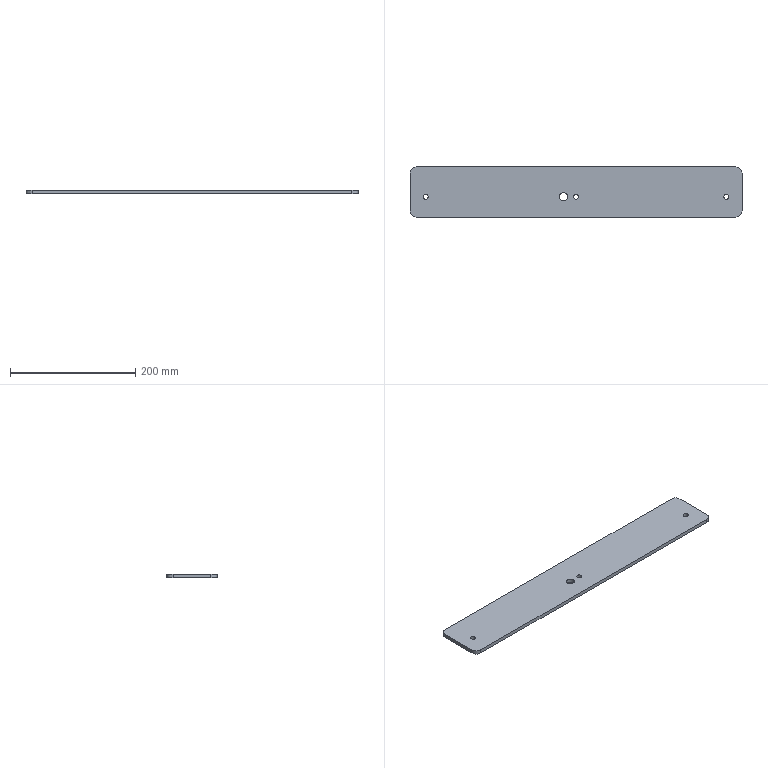Part | SolidWorks | features FlatPattern 1, SMBaseFlange 1, SheetMetal 1 | 1 solid | 18 faces | box 530 x 80 x 6 mm | volume 252184 mm3 | cylinder 12 | plane 6 | commonest cylinder face diameters 8 x6 20 x4 13 x2
STEP:
#1=CARTESIAN_POINT('',(-234.,927.5,6.));
#2=VERTEX_POINT('',#1);
#3=CARTESIAN_POINT('',(-226.,927.5,6.));
#4=VERTEX_POINT('',#3);
#5=CARTESIAN_POINT('',(-230.,927.5,6.));
#6=DIRECTION('',(0.,0.,1.));
#7=DIRECTION('',(1.,0.,0.));
#8=AXIS2_PLACEMENT_3D('',#5,#6,#7);
#9=CIRCLE('',#8,4.);
#10=EDGE_CURVE('',#2,#4,#9,.T.);
#11=ORIENTED_EDGE('',*,*,#10,.T.);
#12=CARTESIAN_POINT('',(-226.,927.5,0.));
#13=VERTEX_POINT('',#12);
#14=CARTESIAN_POINT('',(-226.,927.5,6.));
#15=DIRECTION('',(0.,0.,-1.));
#16=VECTOR('',#15,1000.);
#17=LINE('',#14,#16);
#18=EDGE_CURVE('',#4,#13,#17,.T.);
#19=ORIENTED_EDGE('',*,*,#18,.T.);
#20=CARTESIAN_POINT('',(-234.,927.5,0.));
#21=VERTEX_POINT('',#20);
#22=CARTESIAN_POINT('',(-230.,927.5,0.));
#23=DIRECTION('',(0.,0.,1.));
#24=DIRECTION('',(1.,0.,0.));
#25=AXIS2_PLACEMENT_3D('',#22,#23,#24);
#26=CIRCLE('',#25,4.);
#27=EDGE_CURVE('',#21,#13,#26,.T.);
#28=ORIENTED_EDGE('',*,*,#27,.F.);
#29=CARTESIAN_POINT('',(-234.,927.5,6.));
#30=DIRECTION('',(0.,0.,-1.));
#31=VECTOR('',#30,1000.);
#32=LINE('',#29,#31);
#33=EDGE_CURVE('',#2,#21,#32,.T.);
#34=ORIENTED_EDGE('',*,*,#33,.F.);
#35=EDGE_LOOP('',(#11,#19,#28,#34));
#36=FACE_OUTER_BOUND('',#35,.T.);
#37=CARTESIAN_POINT('',(-230.,927.5,6.));
#38=DIRECTION('',(0.,0.,-1.));
#39=DIRECTION('',(-1.,0.,0.));
#40=AXIS2_PLACEMENT_3D('',#37,#38,#39);
#41=CYLINDRICAL_SURFACE('',#40,4.);
#42=ADVANCED_FACE('',(#36),#41,.F.);
#43=CARTESIAN_POINT('',(-16.5,927.5,6.));
#44=VERTEX_POINT('',#43);
#45=CARTESIAN_POINT('',(-3.5,927.5,6.));
#46=VERTEX_POINT('',#45);
#47=CARTESIAN_POINT('',(-10.,927.5,6.));
#48=DIRECTION('',(0.,0.,1.));
#49=DIRECTION('',(1.,0.,0.));
#50=AXIS2_PLACEMENT_3D('',#47,#48,#49);
#51=CIRCLE('',#50,6.5);
#52=EDGE_CURVE('',#44,#46,#51,.T.);
#53=ORIENTED_EDGE('',*,*,#52,.T.);
#54=CARTESIAN_POINT('',(-3.5,927.5,0.));
#55=VERTEX_POINT('',#54);
#56=CARTESIAN_POINT('',(-3.5,927.5,6.));
#57=DIRECTION('',(0.,0.,-1.));
#58=VECTOR('',#57,1000.);
#59=LINE('',#56,#58);
#60=EDGE_CURVE('',#46,#55,#59,.T.);
#61=ORIENTED_EDGE('',*,*,#60,.T.);
#62=CARTESIAN_POINT('',(-16.5,927.5,0.));
#63=VERTEX_POINT('',#62);
#64=CARTESIAN_POINT('',(-10.,927.5,0.));
#65=DIRECTION('',(0.,0.,1.));
#66=DIRECTION('',(1.,0.,0.));
#67=AXIS2_PLACEMENT_3D('',#64,#65,#66);
#68=CIRCLE('',#67,6.5);
#69=EDGE_CURVE('',#63,#55,#68,.T.);
#70=ORIENTED_EDGE('',*,*,#69,.F.);
#71=CARTESIAN_POINT('',(-16.5,927.5,6.));
#72=DIRECTION('',(0.,0.,-1.));
#73=VECTOR('',#72,1000.);
#74=LINE('',#71,#73);
#75=EDGE_CURVE('',#44,#63,#74,.T.);
#76=ORIENTED_EDGE('',*,*,#75,.F.);
#77=EDGE_LOOP('',(#53,#61,#70,#76));
#78=FACE_OUTER_BOUND('',#77,.T.);
#79=CARTESIAN_POINT('',(-10.,927.5,6.));
#80=DIRECTION('',(0.,0.,-1.));
#81=DIRECTION('',(-1.,0.,0.));
#82=AXIS2_PLACEMENT_3D('',#79,#80,#81);
#83=CYLINDRICAL_SURFACE('',#82,6.5);
#84=ADVANCED_FACE('',(#78),#83,.F.);
#85=CARTESIAN_POINT('',(6.,927.5,6.));
#86=VERTEX_POINT('',#85);
#87=CARTESIAN_POINT('',(14.,927.5,6.));
#88=VERTEX_POINT('',#87);
#89=CARTESIAN_POINT('',(10.,927.5,6.));
#90=DIRECTION('',(0.,0.,1.));
#91=DIRECTION('',(1.,0.,0.));
#92=AXIS2_PLACEMENT_3D('',#89,#90,#91);
#93=CIRCLE('',#92,4.);
#94=EDGE_CURVE('',#86,#88,#93,.T.);
#95=ORIENTED_EDGE('',*,*,#94,.T.);
#96=CARTESIAN_POINT('',(14.,927.5,0.));
#97=VERTEX_POINT('',#96);
#98=CARTESIAN_POINT('',(14.,927.5,6.));
#99=DIRECTION('',(0.,0.,-1.));
#100=VECTOR('',#99,1000.);
#101=LINE('',#98,#100);
#102=EDGE_CURVE('',#88,#97,#101,.T.);
#103=ORIENTED_EDGE('',*,*,#102,.T.);
#104=CARTESIAN_POINT('',(6.,927.5,0.));
#105=VERTEX_POINT('',#104);
#106=CARTESIAN_POINT('',(10.,927.5,0.));
#107=DIRECTION('',(0.,0.,1.));
#108=DIRECTION('',(1.,0.,0.));
#109=AXIS2_PLACEMENT_3D('',#106,#107,#108);
#110=CIRCLE('',#109,4.);
#111=EDGE_CURVE('',#105,#97,#110,.T.);
#112=ORIENTED_EDGE('',*,*,#111,.F.);
#113=CARTESIAN_POINT('',(6.,927.5,6.));
#114=DIRECTION('',(0.,0.,-1.));
#115=VECTOR('',#114,1000.);
#116=LINE('',#113,#115);
#117=EDGE_CURVE('',#86,#105,#116,.T.);
#118=ORIENTED_EDGE('',*,*,#117,.F.);
#119=EDGE_LOOP('',(#95,#103,#112,#118));
#120=FACE_OUTER_BOUND('',#119,.T.);
#121=CARTESIAN_POINT('',(10.,927.5,6.));
#122=DIRECTION('',(0.,0.,-1.));
#123=DIRECTION('',(-1.,0.,0.));
#124=AXIS2_PLACEMENT_3D('',#121,#122,#123);
#125=CYLINDRICAL_SURFACE('',#124,4.);
#126=ADVANCED_FACE('',(#120),#125,.F.);
#127=CARTESIAN_POINT('',(246.,927.5,6.));
#128=VERTEX_POINT('',#127);
#129=CARTESIAN_POINT('',(254.,927.5,6.));
#130=VERTEX_POINT('',#129);
#131=CARTESIAN_POINT('',(250.,927.5,6.));
#132=DIRECTION('',(0.,0.,1.));
#133=DIRECTION('',(1.,0.,0.));
#134=AXIS2_PLACEMENT_3D('',#131,#132,#133);
#135=CIRCLE('',#134,4.);
#136=EDGE_CURVE('',#128,#130,#135,.T.);
#137=ORIENTED_EDGE('',*,*,#136,.T.);
#138=CARTESIAN_POINT('',(254.,927.5,0.));
#139=VERTEX_POINT('',#138);
#140=CARTESIAN_POINT('',(254.,927.5,6.));
#141=DIRECTION('',(0.,0.,-1.));
#142=VECTOR('',#141,1000.);
#143=LINE('',#140,#142);
#144=EDGE_CURVE('',#130,#139,#143,.T.);
#145=ORIENTED_EDGE('',*,*,#144,.T.);
#146=CARTESIAN_POINT('',(246.,927.5,0.));
#147=VERTEX_POINT('',#146);
#148=CARTESIAN_POINT('',(250.,927.5,0.));
#149=DIRECTION('',(0.,0.,1.));
#150=DIRECTION('',(1.,0.,0.));
#151=AXIS2_PLACEMENT_3D('',#148,#149,#150);
#152=CIRCLE('',#151,4.);
#153=EDGE_CURVE('',#147,#139,#152,.T.);
#154=ORIENTED_EDGE('',*,*,#153,.F.);
#155=CARTESIAN_POINT('',(246.,927.5,6.));
#156=DIRECTION('',(0.,0.,-1.));
#157=VECTOR('',#156,1000.);
#158=LINE('',#155,#157);
#159=EDGE_CURVE('',#128,#147,#158,.T.);
#160=ORIENTED_EDGE('',*,*,#159,.F.);
#161=EDGE_LOOP('',(#137,#145,#154,#160));
#162=FACE_OUTER_BOUND('',#161,.T.);
#163=CARTESIAN_POINT('',(250.,927.5,6.));
#164=DIRECTION('',(0.,0.,-1.));
#165=DIRECTION('',(-1.,0.,0.));
#166=AXIS2_PLACEMENT_3D('',#163,#164,#165);
#167=CYLINDRICAL_SURFACE('',#166,4.);
#168=ADVANCED_FACE('',(#162),#167,.F.);
#169=CARTESIAN_POINT('',(-255.,905.,6.));
#170=VERTEX_POINT('',#169);
#171=CARTESIAN_POINT('',(-245.,895.,6.));
#172=VERTEX_POINT('',#171);
#173=CARTESIAN_POINT('',(-245.,905.,6.));
#174=DIRECTION('',(0.,0.,1.));
#175=DIRECTION('',(-1.,0.,0.));
#176=AXIS2_PLACEMENT_3D('',#173,#174,#175);
#177=CIRCLE('',#176,10.);
#178=EDGE_CURVE('',#170,#172,#177,.T.);
#179=ORIENTED_EDGE('',*,*,#178,.T.);
#180=CARTESIAN_POINT('',(265.,895.,6.));
#181=VERTEX_POINT('',#180);
#182=CARTESIAN_POINT('',(265.,895.,6.));
#183=DIRECTION('',(1.,0.,0.));
#184=VECTOR('',#183,1000.);
#185=LINE('',#182,#184);
#186=EDGE_CURVE('',#172,#181,#185,.T.);
#187=ORIENTED_EDGE('',*,*,#186,.T.);
#188=CARTESIAN_POINT('',(275.,905.,6.));
#189=VERTEX_POINT('',#188);
#190=CARTESIAN_POINT('',(265.,905.,6.));
#191=DIRECTION('',(0.,0.,1.));
#192=DIRECTION('',(-1.,0.,0.));
#193=AXIS2_PLACEMENT_3D('',#190,#191,#192);
#194=CIRCLE('',#193,10.);
#195=EDGE_CURVE('',#181,#189,#194,.T.);
#196=ORIENTED_EDGE('',*,*,#195,.T.);
#197=CARTESIAN_POINT('',(275.,965.,6.));
#198=VERTEX_POINT('',#197);
#199=CARTESIAN_POINT('',(275.,965.,6.));
#200=DIRECTION('',(0.,1.,0.));
#201=VECTOR('',#200,1000.);
#202=LINE('',#199,#201);
#203=EDGE_CURVE('',#189,#198,#202,.T.);
#204=ORIENTED_EDGE('',*,*,#203,.T.);
#205=CARTESIAN_POINT('',(265.,975.,6.));
#206=VERTEX_POINT('',#205);
#207=CARTESIAN_POINT('',(265.,965.,6.));
#208=DIRECTION('',(0.,0.,1.));
#209=DIRECTION('',(-1.,0.,0.));
#210=AXIS2_PLACEMENT_3D('',#207,#208,#209);
#211=CIRCLE('',#210,10.);
#212=EDGE_CURVE('',#198,#206,#211,.T.);
#213=ORIENTED_EDGE('',*,*,#212,.T.);
#214=CARTESIAN_POINT('',(-245.,975.,6.));
#215=VERTEX_POINT('',#214);
#216=CARTESIAN_POINT('',(265.,975.,6.));
#217=DIRECTION('',(-1.,0.,0.));
#218=VECTOR('',#217,1000.);
#219=LINE('',#216,#218);
#220=EDGE_CURVE('',#206,#215,#219,.T.);
#221=ORIENTED_EDGE('',*,*,#220,.T.);
#222=CARTESIAN_POINT('',(-255.,965.,6.));
#223=VERTEX_POINT('',#222);
#224=CARTESIAN_POINT('',(-245.,965.,6.));
#225=DIRECTION('',(0.,0.,1.));
#226=DIRECTION('',(1.,0.,0.));
#227=AXIS2_PLACEMENT_3D('',#224,#225,#226);
#228=CIRCLE('',#227,10.);
#229=EDGE_CURVE('',#215,#223,#228,.T.);
#230=ORIENTED_EDGE('',*,*,#229,.T.);
#231=CARTESIAN_POINT('',(-255.,965.,6.));
#232=DIRECTION('',(0.,-1.,0.));
#233=VECTOR('',#232,1000.);
#234=LINE('',#231,#233);
#235=EDGE_CURVE('',#223,#170,#234,.T.);
#236=ORIENTED_EDGE('',*,*,#235,.T.);
#237=EDGE_LOOP('',(#179,#187,#196,#204,#213,#221,#230,#236));
#238=FACE_OUTER_BOUND('',#237,.T.);
#239=ORIENTED_EDGE('',*,*,#136,.F.);
#240=CARTESIAN_POINT('',(250.,927.5,6.));
#241=DIRECTION('',(0.,0.,1.));
#242=DIRECTION('',(1.,0.,0.));
#243=AXIS2_PLACEMENT_3D('',#240,#241,#242);
#244=CIRCLE('',#243,4.);
#245=EDGE_CURVE('',#130,#128,#244,.T.);
#246=ORIENTED_EDGE('',*,*,#245,.F.);
#247=EDGE_LOOP('',(#239,#246));
#248=FACE_BOUND('',#247,.T.);
#249=ORIENTED_EDGE('',*,*,#94,.F.);
#250=CARTESIAN_POINT('',(10.,927.5,6.));
#251=DIRECTION('',(0.,0.,1.));
#252=DIRECTION('',(1.,0.,0.));
#253=AXIS2_PLACEMENT_3D('',#250,#251,#252);
#254=CIRCLE('',#253,4.);
#255=EDGE_CURVE('',#88,#86,#254,.T.);
#256=ORIENTED_EDGE('',*,*,#255,.F.);
#257=EDGE_LOOP('',(#249,#256));
#258=FACE_BOUND('',#257,.T.);
#259=ORIENTED_EDGE('',*,*,#52,.F.);
#260=CARTESIAN_POINT('',(-10.,927.5,6.));
#261=DIRECTION('',(0.,0.,1.));
#262=DIRECTION('',(1.,0.,0.));
#263=AXIS2_PLACEMENT_3D('',#260,#261,#262);
#264=CIRCLE('',#263,6.5);
#265=EDGE_CURVE('',#46,#44,#264,.T.);
#266=ORIENTED_EDGE('',*,*,#265,.F.);
#267=EDGE_LOOP('',(#259,#266));
#268=FACE_BOUND('',#267,.T.);
#269=ORIENTED_EDGE('',*,*,#10,.F.);
#270=CARTESIAN_POINT('',(-230.,927.5,6.));
#271=DIRECTION('',(0.,0.,1.));
#272=DIRECTION('',(1.,0.,0.));
#273=AXIS2_PLACEMENT_3D('',#270,#271,#272);
#274=CIRCLE('',#273,4.);
#275=EDGE_CURVE('',#4,#2,#274,.T.);
#276=ORIENTED_EDGE('',*,*,#275,.F.);
#277=EDGE_LOOP('',(#269,#276));
#278=FACE_BOUND('',#277,.T.);
#279=CARTESIAN_POINT('',(-245.,905.,6.));
#280=DIRECTION('',(0.,0.,-1.));
#281=DIRECTION('',(-1.,0.,0.));
#282=AXIS2_PLACEMENT_3D('',#279,#280,#281);
#283=PLANE('',#282);
#284=ADVANCED_FACE('',(#238,#248,#258,#268,#278),#283,.F.);
#285=ORIENTED_EDGE('',*,*,#69,.T.);
#286=CARTESIAN_POINT('',(-10.,927.5,0.));
#287=DIRECTION('',(0.,0.,1.));
#288=DIRECTION('',(1.,0.,0.));
#289=AXIS2_PLACEMENT_3D('',#286,#287,#288);
#290=CIRCLE('',#289,6.5);
#291=EDGE_CURVE('',#55,#63,#290,.T.);
#292=ORIENTED_EDGE('',*,*,#291,.T.);
#293=EDGE_LOOP('',(#285,#292));
#294=FACE_BOUND('',#293,.T.);
#295=ORIENTED_EDGE('',*,*,#153,.T.);
#296=CARTESIAN_POINT('',(250.,927.5,0.));
#297=DIRECTION('',(0.,0.,1.));
#298=DIRECTION('',(1.,0.,0.));
#299=AXIS2_PLACEMENT_3D('',#296,#297,#298);
#300=CIRCLE('',#299,4.);
#301=EDGE_CURVE('',#139,#147,#300,.T.);
#302=ORIENTED_EDGE('',*,*,#301,.T.);
#303=EDGE_LOOP('',(#295,#302));
#304=FACE_BOUND('',#303,.T.);
#305=CARTESIAN_POINT('',(-255.,905.,0.));
#306=VERTEX_POINT('',#305);
#307=CARTESIAN_POINT('',(-245.,895.,0.));
#308=VERTEX_POINT('',#307);
#309=CARTESIAN_POINT('',(-245.,905.,0.));
#310=DIRECTION('',(0.,0.,1.));
#311=DIRECTION('',(-1.,0.,0.));
#312=AXIS2_PLACEMENT_3D('',#309,#310,#311);
#313=CIRCLE('',#312,10.);
#314=EDGE_CURVE('',#306,#308,#313,.T.);
#315=ORIENTED_EDGE('',*,*,#314,.F.);
#316=CARTESIAN_POINT('',(-255.,965.,0.));
#317=VERTEX_POINT('',#316);
#318=CARTESIAN_POINT('',(-255.,965.,0.));
#319=DIRECTION('',(0.,-1.,0.));
#320=VECTOR('',#319,1000.);
#321=LINE('',#318,#320);
#322=EDGE_CURVE('',#317,#306,#321,.T.);
#323=ORIENTED_EDGE('',*,*,#322,.F.);
#324=CARTESIAN_POINT('',(-245.,975.,0.));
#325=VERTEX_POINT('',#324);
#326=CARTESIAN_POINT('',(-245.,965.,0.));
#327=DIRECTION('',(0.,0.,1.));
#328=DIRECTION('',(1.,0.,0.));
#329=AXIS2_PLACEMENT_3D('',#326,#327,#328);
#330=CIRCLE('',#329,10.);
#331=EDGE_CURVE('',#325,#317,#330,.T.);
#332=ORIENTED_EDGE('',*,*,#331,.F.);
#333=CARTESIAN_POINT('',(265.,975.,0.));
#334=VERTEX_POINT('',#333);
#335=CARTESIAN_POINT('',(265.,975.,0.));
#336=DIRECTION('',(-1.,0.,0.));
#337=VECTOR('',#336,1000.);
#338=LINE('',#335,#337);
#339=EDGE_CURVE('',#334,#325,#338,.T.);
#340=ORIENTED_EDGE('',*,*,#339,.F.);
#341=CARTESIAN_POINT('',(275.,965.,0.));
#342=VERTEX_POINT('',#341);
#343=CARTESIAN_POINT('',(265.,965.,0.));
#344=DIRECTION('',(0.,0.,1.));
#345=DIRECTION('',(-1.,0.,0.));
#346=AXIS2_PLACEMENT_3D('',#343,#344,#345);
#347=CIRCLE('',#346,10.);
#348=EDGE_CURVE('',#342,#334,#347,.T.);
#349=ORIENTED_EDGE('',*,*,#348,.F.);
#350=CARTESIAN_POINT('',(275.,905.,0.));
#351=VERTEX_POINT('',#350);
#352=CARTESIAN_POINT('',(275.,965.,0.));
#353=DIRECTION('',(0.,1.,0.));
#354=VECTOR('',#353,1000.);
#355=LINE('',#352,#354);
#356=EDGE_CURVE('',#351,#342,#355,.T.);
#357=ORIENTED_EDGE('',*,*,#356,.F.);
#358=CARTESIAN_POINT('',(265.,895.,0.));
#359=VERTEX_POINT('',#358);
#360=CARTESIAN_POINT('',(265.,905.,0.));
#361=DIRECTION('',(0.,0.,1.));
#362=DIRECTION('',(-1.,0.,0.));
#363=AXIS2_PLACEMENT_3D('',#360,#361,#362);
#364=CIRCLE('',#363,10.);
#365=EDGE_CURVE('',#359,#351,#364,.T.);
#366=ORIENTED_EDGE('',*,*,#365,.F.);
#367=CARTESIAN_POINT('',(265.,895.,0.));
#368=DIRECTION('',(1.,0.,0.));
#369=VECTOR('',#368,1000.);
#370=LINE('',#367,#369);
#371=EDGE_CURVE('',#308,#359,#370,.T.);
#372=ORIENTED_EDGE('',*,*,#371,.F.);
#373=EDGE_LOOP('',(#315,#323,#332,#340,#349,#357,#366,#372));
#374=FACE_OUTER_BOUND('',#373,.T.);
#375=ORIENTED_EDGE('',*,*,#111,.T.);
#376=CARTESIAN_POINT('',(10.,927.5,0.));
#377=DIRECTION('',(0.,0.,1.));
#378=DIRECTION('',(1.,0.,0.));
#379=AXIS2_PLACEMENT_3D('',#376,#377,#378);
#380=CIRCLE('',#379,4.);
#381=EDGE_CURVE('',#97,#105,#380,.T.);
#382=ORIENTED_EDGE('',*,*,#381,.T.);
#383=EDGE_LOOP('',(#375,#382));
#384=FACE_BOUND('',#383,.T.);
#385=ORIENTED_EDGE('',*,*,#27,.T.);
#386=CARTESIAN_POINT('',(-230.,927.5,0.));
#387=DIRECTION('',(0.,0.,1.));
#388=DIRECTION('',(1.,0.,0.));
#389=AXIS2_PLACEMENT_3D('',#386,#387,#388);
#390=CIRCLE('',#389,4.);
#391=EDGE_CURVE('',#13,#21,#390,.T.);
#392=ORIENTED_EDGE('',*,*,#391,.T.);
#393=EDGE_LOOP('',(#385,#392));
#394=FACE_BOUND('',#393,.T.);
#395=CARTESIAN_POINT('',(-245.,905.,0.));
#396=DIRECTION('',(0.,0.,-1.));
#397=DIRECTION('',(-1.,0.,0.));
#398=AXIS2_PLACEMENT_3D('',#395,#396,#397);
#399=PLANE('',#398);
#400=ADVANCED_FACE('',(#294,#304,#374,#384,#394),#399,.T.);
#401=ORIENTED_EDGE('',*,*,#314,.T.);
#402=CARTESIAN_POINT('',(-245.,895.,6.));
#403=DIRECTION('',(0.,0.,-1.));
#404=VECTOR('',#403,1000.);
#405=LINE('',#402,#404);
#406=EDGE_CURVE('',#172,#308,#405,.T.);
#407=ORIENTED_EDGE('',*,*,#406,.F.);
#408=ORIENTED_EDGE('',*,*,#178,.F.);
#409=CARTESIAN_POINT('',(-255.,905.,6.));
#410=DIRECTION('',(0.,0.,-1.));
#411=VECTOR('',#410,1000.);
#412=LINE('',#409,#411);
#413=EDGE_CURVE('',#170,#306,#412,.T.);
#414=ORIENTED_EDGE('',*,*,#413,.T.);
#415=EDGE_LOOP('',(#401,#407,#408,#414));
#416=FACE_OUTER_BOUND('',#415,.T.);
#417=CARTESIAN_POINT('',(-245.,905.,6.));
#418=DIRECTION('',(0.,0.,-1.));
#419=DIRECTION('',(-1.,0.,0.));
#420=AXIS2_PLACEMENT_3D('',#417,#418,#419);
#421=CYLINDRICAL_SURFACE('',#420,10.);
#422=ADVANCED_FACE('',(#416),#421,.T.);
#423=ORIENTED_EDGE('',*,*,#371,.T.);
#424=CARTESIAN_POINT('',(265.,895.,6.));
#425=DIRECTION('',(0.,0.,-1.));
#426=VECTOR('',#425,1000.);
#427=LINE('',#424,#426);
#428=EDGE_CURVE('',#181,#359,#427,.T.);
#429=ORIENTED_EDGE('',*,*,#428,.F.);
#430=ORIENTED_EDGE('',*,*,#186,.F.);
#431=ORIENTED_EDGE('',*,*,#406,.T.);
#432=EDGE_LOOP('',(#423,#429,#430,#431));
#433=FACE_OUTER_BOUND('',#432,.T.);
#434=CARTESIAN_POINT('',(265.,895.,6.));
#435=DIRECTION('',(0.,1.,0.));
#436=DIRECTION('',(-1.,0.,0.));
#437=AXIS2_PLACEMENT_3D('',#434,#435,#436);
#438=PLANE('',#437);
#439=ADVANCED_FACE('',(#433),#438,.F.);
#440=ORIENTED_EDGE('',*,*,#365,.T.);
#441=CARTESIAN_POINT('',(275.,905.,6.));
#442=DIRECTION('',(0.,0.,-1.));
#443=VECTOR('',#442,1000.);
#444=LINE('',#441,#443);
#445=EDGE_CURVE('',#189,#351,#444,.T.);
#446=ORIENTED_EDGE('',*,*,#445,.F.);
#447=ORIENTED_EDGE('',*,*,#195,.F.);
#448=ORIENTED_EDGE('',*,*,#428,.T.);
#449=EDGE_LOOP('',(#440,#446,#447,#448));
#450=FACE_OUTER_BOUND('',#449,.T.);
#451=CARTESIAN_POINT('',(265.,905.,6.));
#452=DIRECTION('',(0.,0.,-1.));
#453=DIRECTION('',(-1.,0.,0.));
#454=AXIS2_PLACEMENT_3D('',#451,#452,#453);
#455=CYLINDRICAL_SURFACE('',#454,10.);
#456=ADVANCED_FACE('',(#450),#455,.T.);
#457=ORIENTED_EDGE('',*,*,#356,.T.);
#458=CARTESIAN_POINT('',(275.,965.,6.));
#459=DIRECTION('',(0.,0.,-1.));
#460=VECTOR('',#459,1000.);
#461=LINE('',#458,#460);
#462=EDGE_CURVE('',#198,#342,#461,.T.);
#463=ORIENTED_EDGE('',*,*,#462,.F.);
#464=ORIENTED_EDGE('',*,*,#203,.F.);
#465=ORIENTED_EDGE('',*,*,#445,.T.);
#466=EDGE_LOOP('',(#457,#463,#464,#465));
#467=FACE_OUTER_BOUND('',#466,.T.);
#468=CARTESIAN_POINT('',(275.,965.,6.));
#469=DIRECTION('',(-1.,0.,0.));
#470=DIRECTION('',(0.,-1.,0.));
#471=AXIS2_PLACEMENT_3D('',#468,#469,#470);
#472=PLANE('',#471);
#473=ADVANCED_FACE('',(#467),#472,.F.);
#474=ORIENTED_EDGE('',*,*,#348,.T.);
#475=CARTESIAN_POINT('',(265.,975.,6.));
#476=DIRECTION('',(0.,0.,-1.));
#477=VECTOR('',#476,1000.);
#478=LINE('',#475,#477);
#479=EDGE_CURVE('',#206,#334,#478,.T.);
#480=ORIENTED_EDGE('',*,*,#479,.F.);
#481=ORIENTED_EDGE('',*,*,#212,.F.);
#482=ORIENTED_EDGE('',*,*,#462,.T.);
#483=EDGE_LOOP('',(#474,#480,#481,#482));
#484=FACE_OUTER_BOUND('',#483,.T.);
#485=CARTESIAN_POINT('',(265.,965.,6.));
#486=DIRECTION('',(0.,0.,-1.));
#487=DIRECTION('',(-1.,0.,0.));
#488=AXIS2_PLACEMENT_3D('',#485,#486,#487);
#489=CYLINDRICAL_SURFACE('',#488,10.);
#490=ADVANCED_FACE('',(#484),#489,.T.);
#491=ORIENTED_EDGE('',*,*,#339,.T.);
#492=CARTESIAN_POINT('',(-245.,975.,6.));
#493=DIRECTION('',(0.,0.,-1.));
#494=VECTOR('',#493,1000.);
#495=LINE('',#492,#494);
#496=EDGE_CURVE('',#215,#325,#495,.T.);
#497=ORIENTED_EDGE('',*,*,#496,.F.);
#498=ORIENTED_EDGE('',*,*,#220,.F.);
#499=ORIENTED_EDGE('',*,*,#479,.T.);
#500=EDGE_LOOP('',(#491,#497,#498,#499));
#501=FACE_OUTER_BOUND('',#500,.T.);
#502=CARTESIAN_POINT('',(265.,975.,6.));
#503=DIRECTION('',(0.,-1.,0.));
#504=DIRECTION('',(0.,0.,-1.));
#505=AXIS2_PLACEMENT_3D('',#502,#503,#504);
#506=PLANE('',#505);
#507=ADVANCED_FACE('',(#501),#506,.F.);
#508=ORIENTED_EDGE('',*,*,#331,.T.);
#509=CARTESIAN_POINT('',(-255.,965.,6.));
#510=DIRECTION('',(0.,0.,-1.));
#511=VECTOR('',#510,1000.);
#512=LINE('',#509,#511);
#513=EDGE_CURVE('',#223,#317,#512,.T.);
#514=ORIENTED_EDGE('',*,*,#513,.F.);
#515=ORIENTED_EDGE('',*,*,#229,.F.);
#516=ORIENTED_EDGE('',*,*,#496,.T.);
#517=EDGE_LOOP('',(#508,#514,#515,#516));
#518=FACE_OUTER_BOUND('',#517,.T.);
#519=CARTESIAN_POINT('',(-245.,965.,6.));
#520=DIRECTION('',(0.,0.,-1.));
#521=DIRECTION('',(-1.,0.,0.));
#522=AXIS2_PLACEMENT_3D('',#519,#520,#521);
#523=CYLINDRICAL_SURFACE('',#522,10.);
#524=ADVANCED_FACE('',(#518),#523,.T.);
#525=ORIENTED_EDGE('',*,*,#322,.T.);
#526=ORIENTED_EDGE('',*,*,#413,.F.);
#527=ORIENTED_EDGE('',*,*,#235,.F.);
#528=ORIENTED_EDGE('',*,*,#513,.T.);
#529=EDGE_LOOP('',(#525,#526,#527,#528));
#530=FACE_OUTER_BOUND('',#529,.T.);
#531=CARTESIAN_POINT('',(-255.,965.,6.));
#532=DIRECTION('',(1.,0.,0.));
#533=DIRECTION('',(0.,1.,0.));
#534=AXIS2_PLACEMENT_3D('',#531,#532,#533);
#535=PLANE('',#534);
#536=ADVANCED_FACE('',(#530),#535,.F.);
#537=ORIENTED_EDGE('',*,*,#144,.F.);
#538=ORIENTED_EDGE('',*,*,#245,.T.);
#539=ORIENTED_EDGE('',*,*,#159,.T.);
#540=ORIENTED_EDGE('',*,*,#301,.F.);
#541=EDGE_LOOP('',(#537,#538,#539,#540));
#542=FACE_OUTER_BOUND('',#541,.T.);
#543=CARTESIAN_POINT('',(250.,927.5,6.));
#544=DIRECTION('',(0.,0.,-1.));
#545=DIRECTION('',(-1.,0.,0.));
#546=AXIS2_PLACEMENT_3D('',#543,#544,#545);
#547=CYLINDRICAL_SURFACE('',#546,4.);
#548=ADVANCED_FACE('',(#542),#547,.F.);
#549=ORIENTED_EDGE('',*,*,#102,.F.);
#550=ORIENTED_EDGE('',*,*,#255,.T.);
#551=ORIENTED_EDGE('',*,*,#117,.T.);
#552=ORIENTED_EDGE('',*,*,#381,.F.);
#553=EDGE_LOOP('',(#549,#550,#551,#552));
#554=FACE_OUTER_BOUND('',#553,.T.);
#555=CARTESIAN_POINT('',(10.,927.5,6.));
#556=DIRECTION('',(0.,0.,-1.));
#557=DIRECTION('',(-1.,0.,0.));
#558=AXIS2_PLACEMENT_3D('',#555,#556,#557);
#559=CYLINDRICAL_SURFACE('',#558,4.);
#560=ADVANCED_FACE('',(#554),#559,.F.);
#561=ORIENTED_EDGE('',*,*,#60,.F.);
#562=ORIENTED_EDGE('',*,*,#265,.T.);
#563=ORIENTED_EDGE('',*,*,#75,.T.);
#564=ORIENTED_EDGE('',*,*,#291,.F.);
#565=EDGE_LOOP('',(#561,#562,#563,#564));
#566=FACE_OUTER_BOUND('',#565,.T.);
#567=CARTESIAN_POINT('',(-10.,927.5,6.));
#568=DIRECTION('',(0.,0.,-1.));
#569=DIRECTION('',(-1.,0.,0.));
#570=AXIS2_PLACEMENT_3D('',#567,#568,#569);
#571=CYLINDRICAL_SURFACE('',#570,6.5);
#572=ADVANCED_FACE('',(#566),#571,.F.);
#573=ORIENTED_EDGE('',*,*,#18,.F.);
#574=ORIENTED_EDGE('',*,*,#275,.T.);
#575=ORIENTED_EDGE('',*,*,#33,.T.);
#576=ORIENTED_EDGE('',*,*,#391,.F.);
#577=EDGE_LOOP('',(#573,#574,#575,#576));
#578=FACE_OUTER_BOUND('',#577,.T.);
#579=CARTESIAN_POINT('',(-230.,927.5,6.));
#580=DIRECTION('',(0.,0.,-1.));
#581=DIRECTION('',(-1.,0.,0.));
#582=AXIS2_PLACEMENT_3D('',#579,#580,#581);
#583=CYLINDRICAL_SURFACE('',#582,4.);
#584=ADVANCED_FACE('',(#578),#583,.F.);
#585=CLOSED_SHELL('',(#42,#84,#126,#168,#284,#400,#422,#439,#456,#473,#490,#507,#524,#536,#548,#560,#572,#584));
#586=MANIFOLD_SOLID_BREP('',#585);
#587=CARTESIAN_POINT('',(0.,0.,0.));
#588=DIRECTION('',(0.,0.,1.));
#589=DIRECTION('',(1.,0.,0.));
#590=AXIS2_PLACEMENT_3D('',#587,#588,#589);
#591=(LENGTH_UNIT()NAMED_UNIT(*)SI_UNIT(.MILLI.,.METRE.));
#592=UNCERTAINTY_MEASURE_WITH_UNIT(LENGTH_MEASURE(0.00001),#591,'','');
#593=(NAMED_UNIT(*)PLANE_ANGLE_UNIT()SI_UNIT($,.RADIAN.));
#594=(NAMED_UNIT(*)SI_UNIT($,.STERADIAN.)SOLID_ANGLE_UNIT());
#595=(GEOMETRIC_REPRESENTATION_CONTEXT(3)GLOBAL_UNCERTAINTY_ASSIGNED_CONTEXT((#592))GLOBAL_UNIT_ASSIGNED_CONTEXT((#591,#593,#594))REPRESENTATION_CONTEXT('',''));
#596=ADVANCED_BREP_SHAPE_REPRESENTATION('',(#586,#590),#595);